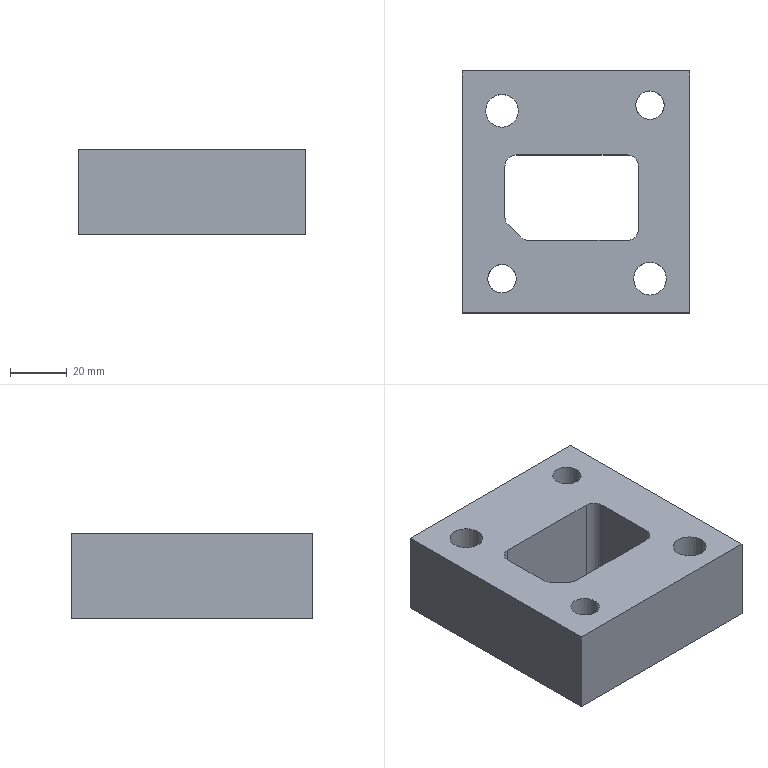Part | NX | features 7 2 | 1 solid | 28 faces | box 80 x 85 x 30 mm | volume 147731 mm3 | plane 15 | cylinder 13 | commonest cylinder face diameters 8 x5 10.001 x2 10.31 x2 11.5 x2 18 x2
STEP:
#1=CARTESIAN_POINT('',(3175.438,56.938,91.));
#2=VERTEX_POINT('',#1);
#3=CARTESIAN_POINT('',(3214.438,56.938,91.));
#4=VERTEX_POINT('',#3);
#5=CARTESIAN_POINT('',(3186.438,56.938,91.));
#6=DIRECTION('',(1.,0.,0.));
#7=VECTOR('',#6,1000.);
#8=LINE('',#5,#7);
#9=EDGE_CURVE('',#2,#4,#8,.T.);
#10=ORIENTED_EDGE('',*,*,#9,.T.);
#11=CARTESIAN_POINT('',(3218.438,52.938,91.));
#12=VERTEX_POINT('',#11);
#13=CARTESIAN_POINT('',(3214.438,52.938,91.));
#14=DIRECTION('',(0.,0.,1.));
#15=DIRECTION('',(0.,1.,0.));
#16=AXIS2_PLACEMENT_3D('',#13,#14,#15);
#17=CIRCLE('',#16,4.);
#18=EDGE_CURVE('',#12,#4,#17,.T.);
#19=ORIENTED_EDGE('',*,*,#18,.F.);
#20=CARTESIAN_POINT('',(3218.438,30.938,91.));
#21=VERTEX_POINT('',#20);
#22=CARTESIAN_POINT('',(3218.438,41.938,91.));
#23=DIRECTION('',(0.,-1.,0.));
#24=VECTOR('',#23,1000.);
#25=LINE('',#22,#24);
#26=EDGE_CURVE('',#12,#21,#25,.T.);
#27=ORIENTED_EDGE('',*,*,#26,.T.);
#28=CARTESIAN_POINT('',(3214.438,26.938,91.));
#29=VERTEX_POINT('',#28);
#30=CARTESIAN_POINT('',(3214.438,30.938,91.));
#31=DIRECTION('',(0.,0.,1.));
#32=DIRECTION('',(0.,1.,0.));
#33=AXIS2_PLACEMENT_3D('',#30,#31,#32);
#34=CIRCLE('',#33,4.);
#35=EDGE_CURVE('',#29,#21,#34,.T.);
#36=ORIENTED_EDGE('',*,*,#35,.F.);
#37=CARTESIAN_POINT('',(3179.731,26.938,91.));
#38=VERTEX_POINT('',#37);
#39=CARTESIAN_POINT('',(3186.438,26.938,91.));
#40=DIRECTION('',(-1.,0.,0.));
#41=VECTOR('',#40,1000.);
#42=LINE('',#39,#41);
#43=EDGE_CURVE('',#29,#38,#42,.T.);
#44=ORIENTED_EDGE('',*,*,#43,.T.);
#45=CARTESIAN_POINT('',(3176.902,28.11,91.));
#46=VERTEX_POINT('',#45);
#47=CARTESIAN_POINT('',(3179.731,30.938,91.));
#48=DIRECTION('',(0.,0.,1.));
#49=DIRECTION('',(0.,-1.,0.));
#50=AXIS2_PLACEMENT_3D('',#47,#48,#49);
#51=CIRCLE('',#50,4.);
#52=EDGE_CURVE('',#46,#38,#51,.T.);
#53=ORIENTED_EDGE('',*,*,#52,.F.);
#54=CARTESIAN_POINT('',(3172.609,32.403,91.));
#55=VERTEX_POINT('',#54);
#56=CARTESIAN_POINT('',(3176.006,29.006,91.));
#57=DIRECTION('',(0.7071,-0.7071,0.));
#58=VECTOR('',#57,1000.);
#59=LINE('',#56,#58);
#60=EDGE_CURVE('',#55,#46,#59,.T.);
#61=ORIENTED_EDGE('',*,*,#60,.F.);
#62=CARTESIAN_POINT('',(3171.438,35.231,91.));
#63=VERTEX_POINT('',#62);
#64=CARTESIAN_POINT('',(3175.438,35.231,91.));
#65=DIRECTION('',(0.,0.,1.));
#66=DIRECTION('',(0.,-1.,0.));
#67=AXIS2_PLACEMENT_3D('',#64,#65,#66);
#68=CIRCLE('',#67,4.);
#69=EDGE_CURVE('',#63,#55,#68,.T.);
#70=ORIENTED_EDGE('',*,*,#69,.F.);
#71=CARTESIAN_POINT('',(3171.438,52.938,91.));
#72=VERTEX_POINT('',#71);
#73=CARTESIAN_POINT('',(3171.438,41.938,91.));
#74=DIRECTION('',(0.,1.,0.));
#75=VECTOR('',#74,1000.);
#76=LINE('',#73,#75);
#77=EDGE_CURVE('',#63,#72,#76,.T.);
#78=ORIENTED_EDGE('',*,*,#77,.T.);
#79=CARTESIAN_POINT('',(3175.438,52.938,91.));
#80=DIRECTION('',(0.,0.,1.));
#81=DIRECTION('',(0.,-1.,0.));
#82=AXIS2_PLACEMENT_3D('',#79,#80,#81);
#83=CIRCLE('',#82,4.);
#84=EDGE_CURVE('',#2,#72,#83,.T.);
#85=ORIENTED_EDGE('',*,*,#84,.F.);
#86=EDGE_LOOP('',(#10,#19,#27,#36,#44,#53,#61,#70,#78,#85));
#87=FACE_BOUND('',#86,.T.);
#88=CARTESIAN_POINT('',(3222.438,79.439,91.));
#89=VERTEX_POINT('',#88);
#90=CARTESIAN_POINT('',(3222.438,74.438,91.));
#91=DIRECTION('',(0.,0.,-1.));
#92=DIRECTION('',(0.,1.,0.));
#93=AXIS2_PLACEMENT_3D('',#90,#91,#92);
#94=CIRCLE('',#93,5.);
#95=EDGE_CURVE('',#89,#89,#94,.T.);
#96=ORIENTED_EDGE('',*,*,#95,.T.);
#97=EDGE_LOOP('',(#96));
#98=FACE_BOUND('',#97,.T.);
#99=CARTESIAN_POINT('',(3170.438,78.188,91.));
#100=VERTEX_POINT('',#99);
#101=CARTESIAN_POINT('',(3170.438,72.438,91.));
#102=DIRECTION('',(0.,0.,1.));
#103=DIRECTION('',(0.,1.,0.));
#104=AXIS2_PLACEMENT_3D('',#101,#102,#103);
#105=CIRCLE('',#104,5.75);
#106=EDGE_CURVE('',#100,#100,#105,.T.);
#107=ORIENTED_EDGE('',*,*,#106,.F.);
#108=EDGE_LOOP('',(#107));
#109=FACE_BOUND('',#108,.T.);
#110=CARTESIAN_POINT('',(3236.438,1.438,91.));
#111=VERTEX_POINT('',#110);
#112=CARTESIAN_POINT('',(3156.438,1.438,91.));
#113=VERTEX_POINT('',#112);
#114=CARTESIAN_POINT('',(3186.438,1.438,91.));
#115=DIRECTION('',(-1.,0.,0.));
#116=VECTOR('',#115,1000.);
#117=LINE('',#114,#116);
#118=EDGE_CURVE('',#111,#113,#117,.T.);
#119=ORIENTED_EDGE('',*,*,#118,.F.);
#120=CARTESIAN_POINT('',(3236.438,86.438,91.));
#121=VERTEX_POINT('',#120);
#122=CARTESIAN_POINT('',(3236.438,41.938,91.));
#123=DIRECTION('',(0.,-1.,0.));
#124=VECTOR('',#123,1000.);
#125=LINE('',#122,#124);
#126=EDGE_CURVE('',#121,#111,#125,.T.);
#127=ORIENTED_EDGE('',*,*,#126,.F.);
#128=CARTESIAN_POINT('',(3156.438,86.438,91.));
#129=VERTEX_POINT('',#128);
#130=CARTESIAN_POINT('',(3186.438,86.438,91.));
#131=DIRECTION('',(1.,0.,0.));
#132=VECTOR('',#131,1000.);
#133=LINE('',#130,#132);
#134=EDGE_CURVE('',#129,#121,#133,.T.);
#135=ORIENTED_EDGE('',*,*,#134,.F.);
#136=CARTESIAN_POINT('',(3156.438,41.938,91.));
#137=DIRECTION('',(0.,1.,0.));
#138=VECTOR('',#137,1000.);
#139=LINE('',#136,#138);
#140=EDGE_CURVE('',#113,#129,#139,.T.);
#141=ORIENTED_EDGE('',*,*,#140,.F.);
#142=EDGE_LOOP('',(#119,#127,#135,#141));
#143=FACE_BOUND('',#142,.T.);
#144=CARTESIAN_POINT('',(3222.438,19.188,91.));
#145=VERTEX_POINT('',#144);
#146=CARTESIAN_POINT('',(3222.438,13.438,91.));
#147=DIRECTION('',(0.,0.,1.));
#148=DIRECTION('',(0.,1.,0.));
#149=AXIS2_PLACEMENT_3D('',#146,#147,#148);
#150=CIRCLE('',#149,5.75);
#151=EDGE_CURVE('',#145,#145,#150,.T.);
#152=ORIENTED_EDGE('',*,*,#151,.F.);
#153=EDGE_LOOP('',(#152));
#154=FACE_BOUND('',#153,.T.);
#155=CARTESIAN_POINT('',(3170.438,18.439,91.));
#156=VERTEX_POINT('',#155);
#157=CARTESIAN_POINT('',(3170.438,13.438,91.));
#158=DIRECTION('',(0.,0.,-1.));
#159=DIRECTION('',(0.,1.,0.));
#160=AXIS2_PLACEMENT_3D('',#157,#158,#159);
#161=CIRCLE('',#160,5.);
#162=EDGE_CURVE('',#156,#156,#161,.T.);
#163=ORIENTED_EDGE('',*,*,#162,.T.);
#164=EDGE_LOOP('',(#163));
#165=FACE_BOUND('',#164,.T.);
#166=CARTESIAN_POINT('',(3186.438,41.938,91.));
#167=DIRECTION('',(0.,0.,1.));
#168=DIRECTION('',(0.,-1.,0.));
#169=AXIS2_PLACEMENT_3D('',#166,#167,#168);
#170=PLANE('',#169);
#171=ADVANCED_FACE('',(#87,#98,#109,#143,#154,#165),#170,.T.);
#172=CARTESIAN_POINT('',(3227.593,74.438,61.));
#173=VERTEX_POINT('',#172);
#174=CARTESIAN_POINT('',(3222.438,74.438,61.));
#175=DIRECTION('',(0.,0.,1.));
#176=DIRECTION('',(1.,0.,0.));
#177=AXIS2_PLACEMENT_3D('',#174,#175,#176);
#178=CIRCLE('',#177,5.155);
#179=EDGE_CURVE('',#173,#173,#178,.T.);
#180=ORIENTED_EDGE('',*,*,#179,.T.);
#181=EDGE_LOOP('',(#180));
#182=FACE_BOUND('',#181,.T.);
#183=CARTESIAN_POINT('',(3175.593,13.438,61.));
#184=VERTEX_POINT('',#183);
#185=CARTESIAN_POINT('',(3170.438,13.438,61.));
#186=DIRECTION('',(0.,0.,1.));
#187=DIRECTION('',(1.,0.,0.));
#188=AXIS2_PLACEMENT_3D('',#185,#186,#187);
#189=CIRCLE('',#188,5.155);
#190=EDGE_CURVE('',#184,#184,#189,.T.);
#191=ORIENTED_EDGE('',*,*,#190,.T.);
#192=EDGE_LOOP('',(#191));
#193=FACE_BOUND('',#192,.T.);
#194=CARTESIAN_POINT('',(3171.438,52.938,61.));
#195=VERTEX_POINT('',#194);
#196=CARTESIAN_POINT('',(3175.438,56.938,61.));
#197=VERTEX_POINT('',#196);
#198=CARTESIAN_POINT('',(3175.438,52.938,61.));
#199=DIRECTION('',(0.,0.,-1.));
#200=DIRECTION('',(0.,1.,0.));
#201=AXIS2_PLACEMENT_3D('',#198,#199,#200);
#202=CIRCLE('',#201,4.);
#203=EDGE_CURVE('',#195,#197,#202,.T.);
#204=ORIENTED_EDGE('',*,*,#203,.F.);
#205=CARTESIAN_POINT('',(3171.438,35.231,61.));
#206=VERTEX_POINT('',#205);
#207=CARTESIAN_POINT('',(3171.438,41.938,61.));
#208=DIRECTION('',(0.,-1.,0.));
#209=VECTOR('',#208,1000.);
#210=LINE('',#207,#209);
#211=EDGE_CURVE('',#195,#206,#210,.T.);
#212=ORIENTED_EDGE('',*,*,#211,.T.);
#213=CARTESIAN_POINT('',(3172.609,32.403,61.));
#214=VERTEX_POINT('',#213);
#215=CARTESIAN_POINT('',(3175.438,35.231,61.));
#216=DIRECTION('',(0.,0.,-1.));
#217=DIRECTION('',(0.,1.,0.));
#218=AXIS2_PLACEMENT_3D('',#215,#216,#217);
#219=CIRCLE('',#218,4.);
#220=EDGE_CURVE('',#214,#206,#219,.T.);
#221=ORIENTED_EDGE('',*,*,#220,.F.);
#222=CARTESIAN_POINT('',(3176.902,28.11,61.));
#223=VERTEX_POINT('',#222);
#224=CARTESIAN_POINT('',(3178.756,26.256,61.));
#225=DIRECTION('',(-0.7071,0.7071,0.));
#226=VECTOR('',#225,1000.);
#227=LINE('',#224,#226);
#228=EDGE_CURVE('',#223,#214,#227,.T.);
#229=ORIENTED_EDGE('',*,*,#228,.F.);
#230=CARTESIAN_POINT('',(3179.731,26.938,61.));
#231=VERTEX_POINT('',#230);
#232=CARTESIAN_POINT('',(3179.731,30.938,61.));
#233=DIRECTION('',(0.,0.,-1.));
#234=DIRECTION('',(0.,1.,0.));
#235=AXIS2_PLACEMENT_3D('',#232,#233,#234);
#236=CIRCLE('',#235,4.);
#237=EDGE_CURVE('',#231,#223,#236,.T.);
#238=ORIENTED_EDGE('',*,*,#237,.F.);
#239=CARTESIAN_POINT('',(3214.438,26.938,61.));
#240=VERTEX_POINT('',#239);
#241=CARTESIAN_POINT('',(3186.438,26.938,61.));
#242=DIRECTION('',(1.,0.,0.));
#243=VECTOR('',#242,1000.);
#244=LINE('',#241,#243);
#245=EDGE_CURVE('',#231,#240,#244,.T.);
#246=ORIENTED_EDGE('',*,*,#245,.T.);
#247=CARTESIAN_POINT('',(3218.438,30.938,61.));
#248=VERTEX_POINT('',#247);
#249=CARTESIAN_POINT('',(3214.438,30.938,61.));
#250=DIRECTION('',(0.,0.,-1.));
#251=DIRECTION('',(0.,-1.,0.));
#252=AXIS2_PLACEMENT_3D('',#249,#250,#251);
#253=CIRCLE('',#252,4.);
#254=EDGE_CURVE('',#248,#240,#253,.T.);
#255=ORIENTED_EDGE('',*,*,#254,.F.);
#256=CARTESIAN_POINT('',(3218.438,52.938,61.));
#257=VERTEX_POINT('',#256);
#258=CARTESIAN_POINT('',(3218.438,41.938,61.));
#259=DIRECTION('',(0.,1.,0.));
#260=VECTOR('',#259,1000.);
#261=LINE('',#258,#260);
#262=EDGE_CURVE('',#248,#257,#261,.T.);
#263=ORIENTED_EDGE('',*,*,#262,.T.);
#264=CARTESIAN_POINT('',(3214.438,56.938,61.));
#265=VERTEX_POINT('',#264);
#266=CARTESIAN_POINT('',(3214.438,52.938,61.));
#267=DIRECTION('',(0.,0.,-1.));
#268=DIRECTION('',(0.,-1.,0.));
#269=AXIS2_PLACEMENT_3D('',#266,#267,#268);
#270=CIRCLE('',#269,4.);
#271=EDGE_CURVE('',#265,#257,#270,.T.);
#272=ORIENTED_EDGE('',*,*,#271,.F.);
#273=CARTESIAN_POINT('',(3186.438,56.938,61.));
#274=DIRECTION('',(-1.,0.,0.));
#275=VECTOR('',#274,1000.);
#276=LINE('',#273,#275);
#277=EDGE_CURVE('',#265,#197,#276,.T.);
#278=ORIENTED_EDGE('',*,*,#277,.T.);
#279=EDGE_LOOP('',(#204,#212,#221,#229,#238,#246,#255,#263,#272,#278));
#280=FACE_BOUND('',#279,.T.);
#281=CARTESIAN_POINT('',(3156.438,86.438,61.));
#282=VERTEX_POINT('',#281);
#283=CARTESIAN_POINT('',(3156.438,1.438,61.));
#284=VERTEX_POINT('',#283);
#285=CARTESIAN_POINT('',(3156.438,41.938,61.));
#286=DIRECTION('',(0.,-1.,0.));
#287=VECTOR('',#286,1000.);
#288=LINE('',#285,#287);
#289=EDGE_CURVE('',#282,#284,#288,.T.);
#290=ORIENTED_EDGE('',*,*,#289,.F.);
#291=CARTESIAN_POINT('',(3236.438,86.438,61.));
#292=VERTEX_POINT('',#291);
#293=CARTESIAN_POINT('',(3186.438,86.438,61.));
#294=DIRECTION('',(-1.,0.,0.));
#295=VECTOR('',#294,1000.);
#296=LINE('',#293,#295);
#297=EDGE_CURVE('',#292,#282,#296,.T.);
#298=ORIENTED_EDGE('',*,*,#297,.F.);
#299=CARTESIAN_POINT('',(3236.438,1.438,61.));
#300=VERTEX_POINT('',#299);
#301=CARTESIAN_POINT('',(3236.438,41.938,61.));
#302=DIRECTION('',(0.,1.,0.));
#303=VECTOR('',#302,1000.);
#304=LINE('',#301,#303);
#305=EDGE_CURVE('',#300,#292,#304,.T.);
#306=ORIENTED_EDGE('',*,*,#305,.F.);
#307=CARTESIAN_POINT('',(3186.438,1.438,61.));
#308=DIRECTION('',(1.,0.,0.));
#309=VECTOR('',#308,1000.);
#310=LINE('',#307,#309);
#311=EDGE_CURVE('',#284,#300,#310,.T.);
#312=ORIENTED_EDGE('',*,*,#311,.F.);
#313=EDGE_LOOP('',(#290,#298,#306,#312));
#314=FACE_BOUND('',#313,.T.);
#315=CARTESIAN_POINT('',(3222.438,4.438,61.));
#316=VERTEX_POINT('',#315);
#317=CARTESIAN_POINT('',(3222.438,13.438,61.));
#318=DIRECTION('',(0.,0.,1.));
#319=DIRECTION('',(0.,-1.,0.));
#320=AXIS2_PLACEMENT_3D('',#317,#318,#319);
#321=CIRCLE('',#320,9.);
#322=EDGE_CURVE('',#316,#316,#321,.T.);
#323=ORIENTED_EDGE('',*,*,#322,.T.);
#324=EDGE_LOOP('',(#323));
#325=FACE_BOUND('',#324,.T.);
#326=CARTESIAN_POINT('',(3170.438,63.438,61.));
#327=VERTEX_POINT('',#326);
#328=CARTESIAN_POINT('',(3170.438,72.438,61.));
#329=DIRECTION('',(0.,0.,1.));
#330=DIRECTION('',(0.,-1.,0.));
#331=AXIS2_PLACEMENT_3D('',#328,#329,#330);
#332=CIRCLE('',#331,9.);
#333=EDGE_CURVE('',#327,#327,#332,.T.);
#334=ORIENTED_EDGE('',*,*,#333,.T.);
#335=EDGE_LOOP('',(#334));
#336=FACE_BOUND('',#335,.T.);
#337=CARTESIAN_POINT('',(3371.438,-135.062,61.));
#338=DIRECTION('',(0.,0.,-1.));
#339=DIRECTION('',(0.,1.,0.));
#340=AXIS2_PLACEMENT_3D('',#337,#338,#339);
#341=PLANE('',#340);
#342=ADVANCED_FACE('',(#182,#193,#280,#314,#325,#336),#341,.T.);
#343=ORIENTED_EDGE('',*,*,#140,.T.);
#344=CARTESIAN_POINT('',(3156.438,86.438,6.933));
#345=DIRECTION('',(0.,0.,-1.));
#346=VECTOR('',#345,1000.);
#347=LINE('',#344,#346);
#348=EDGE_CURVE('',#129,#282,#347,.T.);
#349=ORIENTED_EDGE('',*,*,#348,.T.);
#350=ORIENTED_EDGE('',*,*,#289,.T.);
#351=CARTESIAN_POINT('',(3156.438,1.438,6.933));
#352=DIRECTION('',(0.,0.,-1.));
#353=VECTOR('',#352,1000.);
#354=LINE('',#351,#353);
#355=EDGE_CURVE('',#113,#284,#354,.T.);
#356=ORIENTED_EDGE('',*,*,#355,.F.);
#357=EDGE_LOOP('',(#343,#349,#350,#356));
#358=FACE_BOUND('',#357,.T.);
#359=CARTESIAN_POINT('',(3156.438,41.938,6.933));
#360=DIRECTION('',(-1.,0.,0.));
#361=DIRECTION('',(0.,0.,-1.));
#362=AXIS2_PLACEMENT_3D('',#359,#360,#361);
#363=PLANE('',#362);
#364=ADVANCED_FACE('',(#358),#363,.T.);
#365=ORIENTED_EDGE('',*,*,#134,.T.);
#366=CARTESIAN_POINT('',(3236.438,86.438,6.933));
#367=DIRECTION('',(0.,0.,-1.));
#368=VECTOR('',#367,1000.);
#369=LINE('',#366,#368);
#370=EDGE_CURVE('',#121,#292,#369,.T.);
#371=ORIENTED_EDGE('',*,*,#370,.T.);
#372=ORIENTED_EDGE('',*,*,#297,.T.);
#373=ORIENTED_EDGE('',*,*,#348,.F.);
#374=EDGE_LOOP('',(#365,#371,#372,#373));
#375=FACE_BOUND('',#374,.T.);
#376=CARTESIAN_POINT('',(3186.438,86.438,6.933));
#377=DIRECTION('',(0.,1.,0.));
#378=DIRECTION('',(0.,0.,1.));
#379=AXIS2_PLACEMENT_3D('',#376,#377,#378);
#380=PLANE('',#379);
#381=ADVANCED_FACE('',(#375),#380,.T.);
#382=ORIENTED_EDGE('',*,*,#126,.T.);
#383=CARTESIAN_POINT('',(3236.438,1.438,6.933));
#384=DIRECTION('',(0.,0.,1.));
#385=VECTOR('',#384,1000.);
#386=LINE('',#383,#385);
#387=EDGE_CURVE('',#300,#111,#386,.T.);
#388=ORIENTED_EDGE('',*,*,#387,.F.);
#389=ORIENTED_EDGE('',*,*,#305,.T.);
#390=ORIENTED_EDGE('',*,*,#370,.F.);
#391=EDGE_LOOP('',(#382,#388,#389,#390));
#392=FACE_BOUND('',#391,.T.);
#393=CARTESIAN_POINT('',(3236.438,41.938,6.933));
#394=DIRECTION('',(1.,0.,0.));
#395=DIRECTION('',(0.,0.,1.));
#396=AXIS2_PLACEMENT_3D('',#393,#394,#395);
#397=PLANE('',#396);
#398=ADVANCED_FACE('',(#392),#397,.T.);
#399=ORIENTED_EDGE('',*,*,#311,.T.);
#400=ORIENTED_EDGE('',*,*,#387,.T.);
#401=ORIENTED_EDGE('',*,*,#118,.T.);
#402=ORIENTED_EDGE('',*,*,#355,.T.);
#403=EDGE_LOOP('',(#399,#400,#401,#402));
#404=FACE_BOUND('',#403,.T.);
#405=CARTESIAN_POINT('',(3186.438,1.438,6.933));
#406=DIRECTION('',(0.,-1.,0.));
#407=DIRECTION('',(0.,0.,-1.));
#408=AXIS2_PLACEMENT_3D('',#405,#406,#407);
#409=PLANE('',#408);
#410=ADVANCED_FACE('',(#404),#409,.T.);
#411=ORIENTED_EDGE('',*,*,#151,.T.);
#412=EDGE_LOOP('',(#411));
#413=FACE_BOUND('',#412,.T.);
#414=CARTESIAN_POINT('',(3222.438,19.188,74.));
#415=VERTEX_POINT('',#414);
#416=CARTESIAN_POINT('',(3222.438,13.438,74.));
#417=DIRECTION('',(0.,0.,1.));
#418=DIRECTION('',(0.,1.,0.));
#419=AXIS2_PLACEMENT_3D('',#416,#417,#418);
#420=CIRCLE('',#419,5.75);
#421=EDGE_CURVE('',#415,#415,#420,.T.);
#422=ORIENTED_EDGE('',*,*,#421,.F.);
#423=EDGE_LOOP('',(#422));
#424=FACE_BOUND('',#423,.T.);
#425=CARTESIAN_POINT('',(3222.438,13.438,51.));
#426=DIRECTION('',(0.,0.,1.));
#427=DIRECTION('',(0.,-1.,0.));
#428=AXIS2_PLACEMENT_3D('',#425,#426,#427);
#429=CYLINDRICAL_SURFACE('',#428,5.75);
#430=ADVANCED_FACE('',(#413,#424),#429,.F.);
#431=ORIENTED_EDGE('',*,*,#421,.T.);
#432=EDGE_LOOP('',(#431));
#433=FACE_BOUND('',#432,.T.);
#434=CARTESIAN_POINT('',(3222.438,22.438,74.));
#435=VERTEX_POINT('',#434);
#436=CARTESIAN_POINT('',(3222.438,13.438,74.));
#437=DIRECTION('',(0.,0.,1.));
#438=DIRECTION('',(0.,1.,0.));
#439=AXIS2_PLACEMENT_3D('',#436,#437,#438);
#440=CIRCLE('',#439,9.);
#441=EDGE_CURVE('',#435,#435,#440,.T.);
#442=ORIENTED_EDGE('',*,*,#441,.F.);
#443=EDGE_LOOP('',(#442));
#444=FACE_BOUND('',#443,.T.);
#445=CARTESIAN_POINT('',(3222.438,13.438,74.));
#446=DIRECTION('',(0.,0.,1.));
#447=DIRECTION('',(0.,-1.,0.));
#448=AXIS2_PLACEMENT_3D('',#445,#446,#447);
#449=PLANE('',#448);
#450=ADVANCED_FACE('',(#433,#444),#449,.F.);
#451=ORIENTED_EDGE('',*,*,#441,.T.);
#452=EDGE_LOOP('',(#451));
#453=FACE_BOUND('',#452,.T.);
#454=ORIENTED_EDGE('',*,*,#322,.F.);
#455=EDGE_LOOP('',(#454));
#456=FACE_BOUND('',#455,.T.);
#457=CARTESIAN_POINT('',(3222.438,13.438,56.));
#458=DIRECTION('',(0.,0.,1.));
#459=DIRECTION('',(0.,-1.,0.));
#460=AXIS2_PLACEMENT_3D('',#457,#458,#459);
#461=CYLINDRICAL_SURFACE('',#460,9.);
#462=ADVANCED_FACE('',(#453,#456),#461,.F.);
#463=CARTESIAN_POINT('',(3175.438,13.438,71.));
#464=VERTEX_POINT('',#463);
#465=CARTESIAN_POINT('',(3170.438,13.438,71.));
#466=DIRECTION('',(0.,0.,-1.));
#467=DIRECTION('',(1.,0.,0.));
#468=AXIS2_PLACEMENT_3D('',#465,#466,#467);
#469=CIRCLE('',#468,5.);
#470=EDGE_CURVE('',#464,#464,#469,.T.);
#471=ORIENTED_EDGE('',*,*,#470,.T.);
#472=EDGE_LOOP('',(#471));
#473=FACE_BOUND('',#472,.T.);
#474=ORIENTED_EDGE('',*,*,#162,.F.);
#475=EDGE_LOOP('',(#474));
#476=FACE_BOUND('',#475,.T.);
#477=CARTESIAN_POINT('',(3170.438,13.438,621.));
#478=DIRECTION('',(0.,0.,-1.));
#479=DIRECTION('',(0.,1.,0.));
#480=AXIS2_PLACEMENT_3D('',#477,#478,#479);
#481=CYLINDRICAL_SURFACE('',#480,5.);
#482=ADVANCED_FACE('',(#473,#476),#481,.F.);
#483=ORIENTED_EDGE('',*,*,#106,.T.);
#484=EDGE_LOOP('',(#483));
#485=FACE_BOUND('',#484,.T.);
#486=CARTESIAN_POINT('',(3170.438,78.188,74.));
#487=VERTEX_POINT('',#486);
#488=CARTESIAN_POINT('',(3170.438,72.438,74.));
#489=DIRECTION('',(0.,0.,1.));
#490=DIRECTION('',(0.,1.,0.));
#491=AXIS2_PLACEMENT_3D('',#488,#489,#490);
#492=CIRCLE('',#491,5.75);
#493=EDGE_CURVE('',#487,#487,#492,.T.);
#494=ORIENTED_EDGE('',*,*,#493,.F.);
#495=EDGE_LOOP('',(#494));
#496=FACE_BOUND('',#495,.T.);
#497=CARTESIAN_POINT('',(3170.438,72.438,51.));
#498=DIRECTION('',(0.,0.,1.));
#499=DIRECTION('',(0.,-1.,0.));
#500=AXIS2_PLACEMENT_3D('',#497,#498,#499);
#501=CYLINDRICAL_SURFACE('',#500,5.75);
#502=ADVANCED_FACE('',(#485,#496),#501,.F.);
#503=ORIENTED_EDGE('',*,*,#493,.T.);
#504=EDGE_LOOP('',(#503));
#505=FACE_BOUND('',#504,.T.);
#506=CARTESIAN_POINT('',(3170.438,81.438,74.));
#507=VERTEX_POINT('',#506);
#508=CARTESIAN_POINT('',(3170.438,72.438,74.));
#509=DIRECTION('',(0.,0.,1.));
#510=DIRECTION('',(0.,1.,0.));
#511=AXIS2_PLACEMENT_3D('',#508,#509,#510);
#512=CIRCLE('',#511,9.);
#513=EDGE_CURVE('',#507,#507,#512,.T.);
#514=ORIENTED_EDGE('',*,*,#513,.F.);
#515=EDGE_LOOP('',(#514));
#516=FACE_BOUND('',#515,.T.);
#517=CARTESIAN_POINT('',(3170.438,72.438,74.));
#518=DIRECTION('',(0.,0.,1.));
#519=DIRECTION('',(0.,-1.,0.));
#520=AXIS2_PLACEMENT_3D('',#517,#518,#519);
#521=PLANE('',#520);
#522=ADVANCED_FACE('',(#505,#516),#521,.F.);
#523=ORIENTED_EDGE('',*,*,#513,.T.);
#524=EDGE_LOOP('',(#523));
#525=FACE_BOUND('',#524,.T.);
#526=ORIENTED_EDGE('',*,*,#333,.F.);
#527=EDGE_LOOP('',(#526));
#528=FACE_BOUND('',#527,.T.);
#529=CARTESIAN_POINT('',(3170.438,72.438,56.));
#530=DIRECTION('',(0.,0.,1.));
#531=DIRECTION('',(0.,-1.,0.));
#532=AXIS2_PLACEMENT_3D('',#529,#530,#531);
#533=CYLINDRICAL_SURFACE('',#532,9.);
#534=ADVANCED_FACE('',(#525,#528),#533,.F.);
#535=CARTESIAN_POINT('',(3227.438,74.438,71.));
#536=VERTEX_POINT('',#535);
#537=CARTESIAN_POINT('',(3222.438,74.438,71.));
#538=DIRECTION('',(0.,0.,-1.));
#539=DIRECTION('',(1.,0.,0.));
#540=AXIS2_PLACEMENT_3D('',#537,#538,#539);
#541=CIRCLE('',#540,5.);
#542=EDGE_CURVE('',#536,#536,#541,.T.);
#543=ORIENTED_EDGE('',*,*,#542,.T.);
#544=EDGE_LOOP('',(#543));
#545=FACE_BOUND('',#544,.T.);
#546=ORIENTED_EDGE('',*,*,#95,.F.);
#547=EDGE_LOOP('',(#546));
#548=FACE_BOUND('',#547,.T.);
#549=CARTESIAN_POINT('',(3222.438,74.438,621.));
#550=DIRECTION('',(0.,0.,-1.));
#551=DIRECTION('',(0.,1.,0.));
#552=AXIS2_PLACEMENT_3D('',#549,#550,#551);
#553=CYLINDRICAL_SURFACE('',#552,5.);
#554=ADVANCED_FACE('',(#545,#548),#553,.F.);
#555=ORIENTED_EDGE('',*,*,#9,.F.);
#556=CARTESIAN_POINT('',(3175.438,56.938,-5.));
#557=DIRECTION('',(0.,0.,1.));
#558=VECTOR('',#557,1000.);
#559=LINE('',#556,#558);
#560=EDGE_CURVE('',#197,#2,#559,.T.);
#561=ORIENTED_EDGE('',*,*,#560,.F.);
#562=ORIENTED_EDGE('',*,*,#277,.F.);
#563=CARTESIAN_POINT('',(3214.438,56.938,-5.));
#564=DIRECTION('',(0.,0.,1.));
#565=VECTOR('',#564,1000.);
#566=LINE('',#563,#565);
#567=EDGE_CURVE('',#265,#4,#566,.T.);
#568=ORIENTED_EDGE('',*,*,#567,.T.);
#569=EDGE_LOOP('',(#555,#561,#562,#568));
#570=FACE_BOUND('',#569,.T.);
#571=CARTESIAN_POINT('',(3186.438,56.938,-5.));
#572=DIRECTION('',(0.,1.,0.));
#573=DIRECTION('',(0.,0.,1.));
#574=AXIS2_PLACEMENT_3D('',#571,#572,#573);
#575=PLANE('',#574);
#576=ADVANCED_FACE('',(#570),#575,.F.);
#577=ORIENTED_EDGE('',*,*,#26,.F.);
#578=CARTESIAN_POINT('',(3218.438,52.938,-5.));
#579=DIRECTION('',(0.,0.,-1.));
#580=VECTOR('',#579,1000.);
#581=LINE('',#578,#580);
#582=EDGE_CURVE('',#12,#257,#581,.T.);
#583=ORIENTED_EDGE('',*,*,#582,.T.);
#584=ORIENTED_EDGE('',*,*,#262,.F.);
#585=CARTESIAN_POINT('',(3218.438,30.938,-5.));
#586=DIRECTION('',(0.,0.,1.));
#587=VECTOR('',#586,1000.);
#588=LINE('',#585,#587);
#589=EDGE_CURVE('',#248,#21,#588,.T.);
#590=ORIENTED_EDGE('',*,*,#589,.T.);
#591=EDGE_LOOP('',(#577,#583,#584,#590));
#592=FACE_BOUND('',#591,.T.);
#593=CARTESIAN_POINT('',(3218.438,41.938,-5.));
#594=DIRECTION('',(1.,0.,0.));
#595=DIRECTION('',(0.,0.,1.));
#596=AXIS2_PLACEMENT_3D('',#593,#594,#595);
#597=PLANE('',#596);
#598=ADVANCED_FACE('',(#592),#597,.F.);
#599=ORIENTED_EDGE('',*,*,#245,.F.);
#600=CARTESIAN_POINT('',(3179.731,26.938,-5.));
#601=DIRECTION('',(0.,0.,-1.));
#602=VECTOR('',#601,1000.);
#603=LINE('',#600,#602);
#604=EDGE_CURVE('',#38,#231,#603,.T.);
#605=ORIENTED_EDGE('',*,*,#604,.F.);
#606=ORIENTED_EDGE('',*,*,#43,.F.);
#607=CARTESIAN_POINT('',(3214.438,26.938,-5.));
#608=DIRECTION('',(0.,0.,-1.));
#609=VECTOR('',#608,1000.);
#610=LINE('',#607,#609);
#611=EDGE_CURVE('',#29,#240,#610,.T.);
#612=ORIENTED_EDGE('',*,*,#611,.T.);
#613=EDGE_LOOP('',(#599,#605,#606,#612));
#614=FACE_BOUND('',#613,.T.);
#615=CARTESIAN_POINT('',(3186.438,26.938,-5.));
#616=DIRECTION('',(0.,-1.,0.));
#617=DIRECTION('',(0.,0.,-1.));
#618=AXIS2_PLACEMENT_3D('',#615,#616,#617);
#619=PLANE('',#618);
#620=ADVANCED_FACE('',(#614),#619,.F.);
#621=ORIENTED_EDGE('',*,*,#254,.T.);
#622=ORIENTED_EDGE('',*,*,#611,.F.);
#623=ORIENTED_EDGE('',*,*,#35,.T.);
#624=ORIENTED_EDGE('',*,*,#589,.F.);
#625=EDGE_LOOP('',(#621,#622,#623,#624));
#626=FACE_BOUND('',#625,.T.);
#627=CARTESIAN_POINT('',(3214.438,30.938,-5.));
#628=DIRECTION('',(0.,0.,-1.));
#629=DIRECTION('',(0.,-1.,0.));
#630=AXIS2_PLACEMENT_3D('',#627,#628,#629);
#631=CYLINDRICAL_SURFACE('',#630,4.);
#632=ADVANCED_FACE('',(#626),#631,.F.);
#633=ORIENTED_EDGE('',*,*,#271,.T.);
#634=ORIENTED_EDGE('',*,*,#582,.F.);
#635=ORIENTED_EDGE('',*,*,#18,.T.);
#636=ORIENTED_EDGE('',*,*,#567,.F.);
#637=EDGE_LOOP('',(#633,#634,#635,#636));
#638=FACE_BOUND('',#637,.T.);
#639=CARTESIAN_POINT('',(3214.438,52.938,-5.));
#640=DIRECTION('',(0.,0.,-1.));
#641=DIRECTION('',(0.,-1.,0.));
#642=AXIS2_PLACEMENT_3D('',#639,#640,#641);
#643=CYLINDRICAL_SURFACE('',#642,4.);
#644=ADVANCED_FACE('',(#638),#643,.F.);
#645=ORIENTED_EDGE('',*,*,#77,.F.);
#646=CARTESIAN_POINT('',(3171.438,35.231,-5.));
#647=DIRECTION('',(0.,0.,-1.));
#648=VECTOR('',#647,1000.);
#649=LINE('',#646,#648);
#650=EDGE_CURVE('',#63,#206,#649,.T.);
#651=ORIENTED_EDGE('',*,*,#650,.T.);
#652=ORIENTED_EDGE('',*,*,#211,.F.);
#653=CARTESIAN_POINT('',(3171.438,52.938,-5.));
#654=DIRECTION('',(0.,0.,1.));
#655=VECTOR('',#654,1000.);
#656=LINE('',#653,#655);
#657=EDGE_CURVE('',#195,#72,#656,.T.);
#658=ORIENTED_EDGE('',*,*,#657,.T.);
#659=EDGE_LOOP('',(#645,#651,#652,#658));
#660=FACE_BOUND('',#659,.T.);
#661=CARTESIAN_POINT('',(3171.438,41.938,-5.));
#662=DIRECTION('',(-1.,0.,0.));
#663=DIRECTION('',(0.,0.,-1.));
#664=AXIS2_PLACEMENT_3D('',#661,#662,#663);
#665=PLANE('',#664);
#666=ADVANCED_FACE('',(#660),#665,.F.);
#667=ORIENTED_EDGE('',*,*,#60,.T.);
#668=CARTESIAN_POINT('',(3176.902,28.11,-5.));
#669=DIRECTION('',(0.,0.,-1.));
#670=VECTOR('',#669,1000.);
#671=LINE('',#668,#670);
#672=EDGE_CURVE('',#46,#223,#671,.T.);
#673=ORIENTED_EDGE('',*,*,#672,.T.);
#674=ORIENTED_EDGE('',*,*,#228,.T.);
#675=CARTESIAN_POINT('',(3172.609,32.403,-5.));
#676=DIRECTION('',(0.,0.,1.));
#677=VECTOR('',#676,1000.);
#678=LINE('',#675,#677);
#679=EDGE_CURVE('',#214,#55,#678,.T.);
#680=ORIENTED_EDGE('',*,*,#679,.T.);
#681=EDGE_LOOP('',(#667,#673,#674,#680));
#682=FACE_BOUND('',#681,.T.);
#683=CARTESIAN_POINT('',(3178.756,26.256,-5.));
#684=DIRECTION('',(0.7071,0.7071,0.));
#685=DIRECTION('',(0.,0.,1.));
#686=AXIS2_PLACEMENT_3D('',#683,#684,#685);
#687=PLANE('',#686);
#688=ADVANCED_FACE('',(#682),#687,.T.);
#689=ORIENTED_EDGE('',*,*,#237,.T.);
#690=ORIENTED_EDGE('',*,*,#672,.F.);
#691=ORIENTED_EDGE('',*,*,#52,.T.);
#692=ORIENTED_EDGE('',*,*,#604,.T.);
#693=EDGE_LOOP('',(#689,#690,#691,#692));
#694=FACE_BOUND('',#693,.T.);
#695=CARTESIAN_POINT('',(3179.731,30.938,-5.));
#696=DIRECTION('',(0.,0.,1.));
#697=DIRECTION('',(0.,-1.,0.));
#698=AXIS2_PLACEMENT_3D('',#695,#696,#697);
#699=CYLINDRICAL_SURFACE('',#698,4.);
#700=ADVANCED_FACE('',(#694),#699,.F.);
#701=ORIENTED_EDGE('',*,*,#69,.T.);
#702=ORIENTED_EDGE('',*,*,#679,.F.);
#703=ORIENTED_EDGE('',*,*,#220,.T.);
#704=ORIENTED_EDGE('',*,*,#650,.F.);
#705=EDGE_LOOP('',(#701,#702,#703,#704));
#706=FACE_BOUND('',#705,.T.);
#707=CARTESIAN_POINT('',(3175.438,35.231,-5.));
#708=DIRECTION('',(0.,0.,-1.));
#709=DIRECTION('',(0.,1.,0.));
#710=AXIS2_PLACEMENT_3D('',#707,#708,#709);
#711=CYLINDRICAL_SURFACE('',#710,4.);
#712=ADVANCED_FACE('',(#706),#711,.F.);
#713=ORIENTED_EDGE('',*,*,#203,.T.);
#714=ORIENTED_EDGE('',*,*,#560,.T.);
#715=ORIENTED_EDGE('',*,*,#84,.T.);
#716=ORIENTED_EDGE('',*,*,#657,.F.);
#717=EDGE_LOOP('',(#713,#714,#715,#716));
#718=FACE_BOUND('',#717,.T.);
#719=CARTESIAN_POINT('',(3175.438,52.938,-5.));
#720=DIRECTION('',(0.,0.,-1.));
#721=DIRECTION('',(0.,1.,0.));
#722=AXIS2_PLACEMENT_3D('',#719,#720,#721);
#723=CYLINDRICAL_SURFACE('',#722,4.);
#724=ADVANCED_FACE('',(#718),#723,.F.);
#725=CARTESIAN_POINT('',(3175.593,13.438,71.));
#726=VERTEX_POINT('',#725);
#727=CARTESIAN_POINT('',(3170.438,13.438,71.));
#728=DIRECTION('',(0.,0.,-1.));
#729=DIRECTION('',(1.,0.,0.));
#730=AXIS2_PLACEMENT_3D('',#727,#728,#729);
#731=CIRCLE('',#730,5.155);
#732=EDGE_CURVE('',#726,#726,#731,.T.);
#733=ORIENTED_EDGE('',*,*,#732,.T.);
#734=EDGE_LOOP('',(#733));
#735=FACE_BOUND('',#734,.T.);
#736=ORIENTED_EDGE('',*,*,#470,.F.);
#737=EDGE_LOOP('',(#736));
#738=FACE_BOUND('',#737,.T.);
#739=CARTESIAN_POINT('',(3170.438,13.438,71.));
#740=DIRECTION('',(0.,0.,1.));
#741=DIRECTION('',(-1.,0.,0.));
#742=AXIS2_PLACEMENT_3D('',#739,#740,#741);
#743=PLANE('',#742);
#744=ADVANCED_FACE('',(#735,#738),#743,.F.);
#745=ORIENTED_EDGE('',*,*,#732,.F.);
#746=EDGE_LOOP('',(#745));
#747=FACE_BOUND('',#746,.T.);
#748=ORIENTED_EDGE('',*,*,#190,.F.);
#749=EDGE_LOOP('',(#748));
#750=FACE_BOUND('',#749,.T.);
#751=CARTESIAN_POINT('',(3170.438,13.438,61.));
#752=DIRECTION('',(0.,0.,1.));
#753=DIRECTION('',(-1.,0.,0.));
#754=AXIS2_PLACEMENT_3D('',#751,#752,#753);
#755=CYLINDRICAL_SURFACE('',#754,5.155);
#756=ADVANCED_FACE('',(#747,#750),#755,.F.);
#757=CARTESIAN_POINT('',(3227.593,74.438,71.));
#758=VERTEX_POINT('',#757);
#759=CARTESIAN_POINT('',(3222.438,74.438,71.));
#760=DIRECTION('',(0.,0.,-1.));
#761=DIRECTION('',(1.,0.,0.));
#762=AXIS2_PLACEMENT_3D('',#759,#760,#761);
#763=CIRCLE('',#762,5.155);
#764=EDGE_CURVE('',#758,#758,#763,.T.);
#765=ORIENTED_EDGE('',*,*,#764,.T.);
#766=EDGE_LOOP('',(#765));
#767=FACE_BOUND('',#766,.T.);
#768=ORIENTED_EDGE('',*,*,#542,.F.);
#769=EDGE_LOOP('',(#768));
#770=FACE_BOUND('',#769,.T.);
#771=CARTESIAN_POINT('',(3222.438,74.438,71.));
#772=DIRECTION('',(0.,0.,1.));
#773=DIRECTION('',(-1.,0.,0.));
#774=AXIS2_PLACEMENT_3D('',#771,#772,#773);
#775=PLANE('',#774);
#776=ADVANCED_FACE('',(#767,#770),#775,.F.);
#777=ORIENTED_EDGE('',*,*,#764,.F.);
#778=EDGE_LOOP('',(#777));
#779=FACE_BOUND('',#778,.T.);
#780=ORIENTED_EDGE('',*,*,#179,.F.);
#781=EDGE_LOOP('',(#780));
#782=FACE_BOUND('',#781,.T.);
#783=CARTESIAN_POINT('',(3222.438,74.438,61.));
#784=DIRECTION('',(0.,0.,1.));
#785=DIRECTION('',(-1.,0.,0.));
#786=AXIS2_PLACEMENT_3D('',#783,#784,#785);
#787=CYLINDRICAL_SURFACE('',#786,5.155);
#788=ADVANCED_FACE('',(#779,#782),#787,.F.);
#789=CLOSED_SHELL('',(#171,#342,#364,#381,#398,#410,#430,#450,#462,#482,#502,#522,#534,#554,#576,#598,#620,#632,#644,#666,#688,#700,#712,#724,#744,#756,#776,#788));
#790=MANIFOLD_SOLID_BREP('',#789);
#791=(LENGTH_UNIT()NAMED_UNIT(*)SI_UNIT(.MILLI.,.METRE.));
#792=UNCERTAINTY_MEASURE_WITH_UNIT(LENGTH_MEASURE(0.00001),#791,'','');
#793=(NAMED_UNIT(*)PLANE_ANGLE_UNIT()SI_UNIT($,.RADIAN.));
#794=(NAMED_UNIT(*)SI_UNIT($,.STERADIAN.)SOLID_ANGLE_UNIT());
#795=(GEOMETRIC_REPRESENTATION_CONTEXT(3)GLOBAL_UNCERTAINTY_ASSIGNED_CONTEXT((#792))GLOBAL_UNIT_ASSIGNED_CONTEXT((#791,#793,#794))REPRESENTATION_CONTEXT('',''));
#796=ADVANCED_BREP_SHAPE_REPRESENTATION('',(#790),#795);